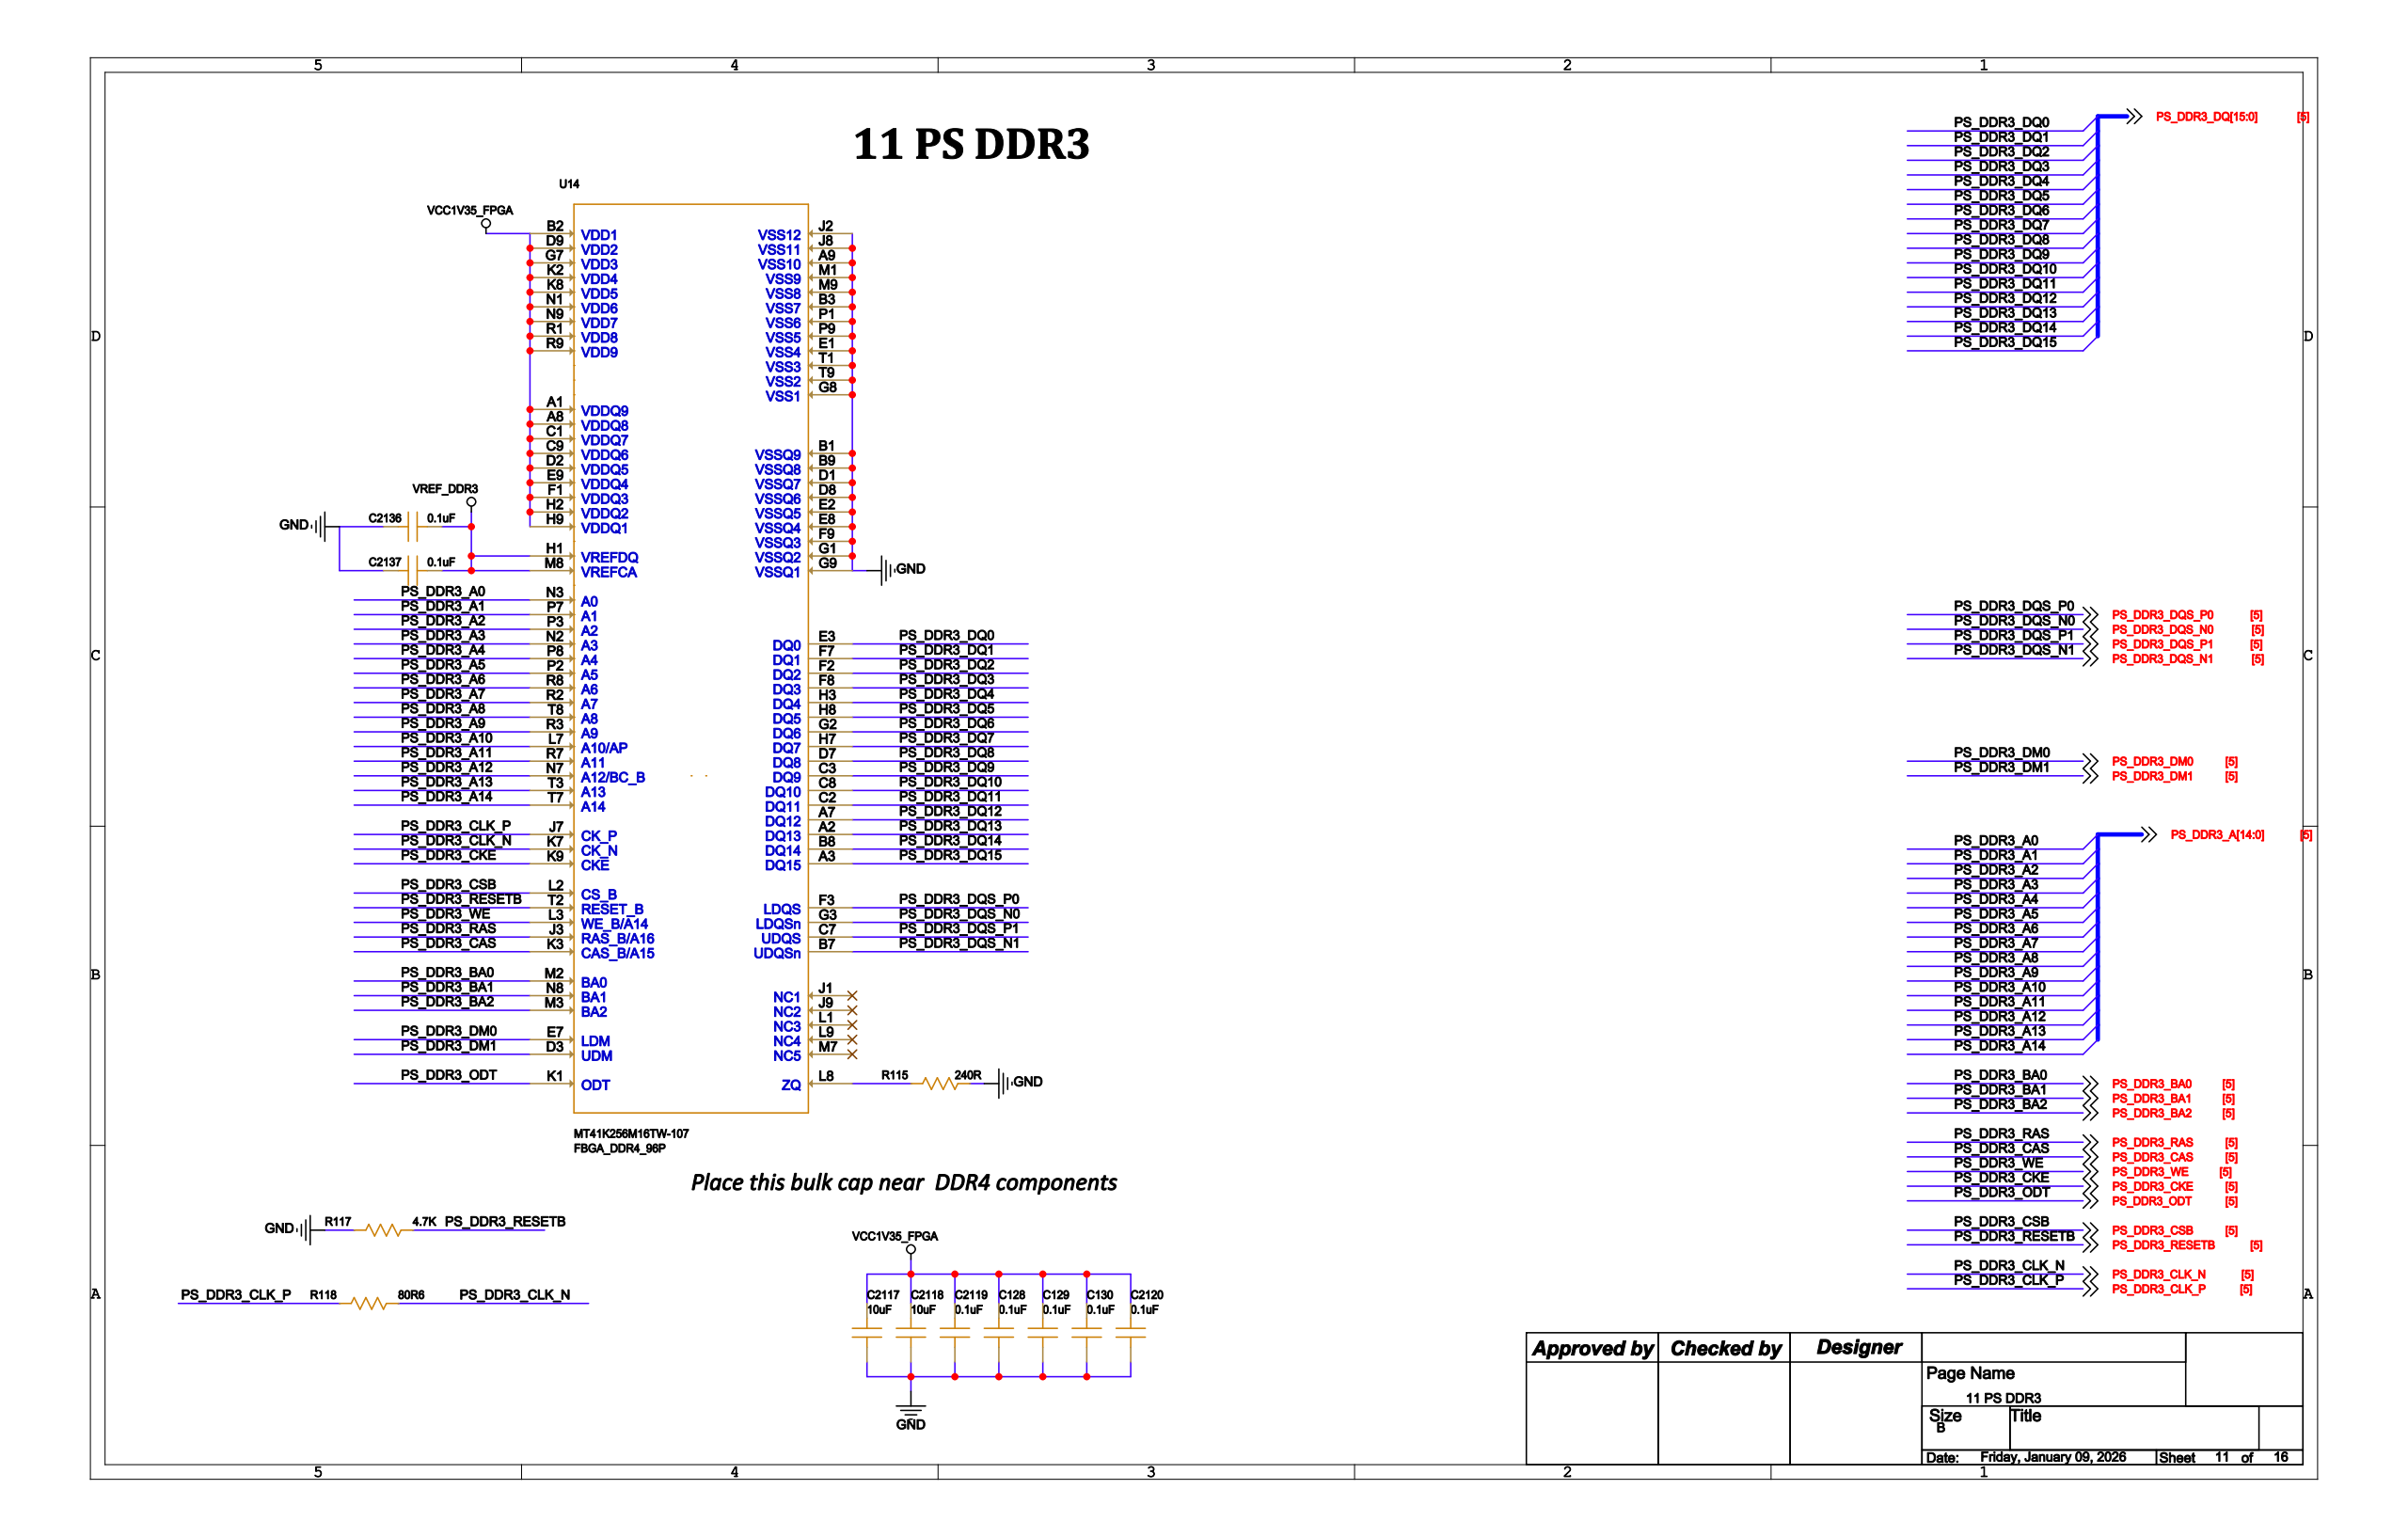Circuit board | Cadence Allegro | 442 parts | 326 nets | one sheet of the schematic
Parts on this sheet (reference | value | footprint):
C128 | 0.1uF | C0201
C129 | 0.1uF | C0201
C130 | 0.1uF | C0201
C2117 | 10uF | C0603
C2118 | 10uF | C0603
C2119 | 0.1uF | C0201
C2120 | 0.1uF | C0201
C2136 | 0.1uF | C0201
C2137 | 0.1uF | C0201
R115 | 240R | R0201
R117 | 4.7K | R0201
R118 | 80R6 | R0201
U14 | MT41K256M16TW-107 | FBGA_DDR4_96P
Nets of these parts (net: part-pin ...):
GND: C128-2 C129-2 C130-2 C2117-2 C2118-2 C2119-2 C2120-2 C2136-2 C2137-2 R115-2 R117-2 U14-A9 U14-B1 U14-B3 U14-B9 U14-D1 U14-D8 U14-E1 U14-E2 U14-E8 U14-F9 U14-G1 U14-G8 U14-G9 U14-J2 U14-J8 U14-M1 U14-M9 U14-P1 U14-P9 U14-T1 U14-T9
PS_DDR3_A0: U14-N3
PS_DDR3_A1: U14-P7
PS_DDR3_A10: U14-L7
PS_DDR3_A11: U14-R7
PS_DDR3_A12: U14-N7
PS_DDR3_A13: U14-T3
PS_DDR3_A14: U14-T7
PS_DDR3_A2: U14-P3
PS_DDR3_A3: U14-N2
PS_DDR3_A4: U14-P8
PS_DDR3_A5: U14-P2
PS_DDR3_A6: U14-R8
PS_DDR3_A7: U14-R2
PS_DDR3_A8: U14-T8
PS_DDR3_A9: U14-R3
PS_DDR3_BA0: U14-M2
PS_DDR3_BA1: U14-N8
PS_DDR3_BA2: U14-M3
PS_DDR3_CAS: U14-K3
PS_DDR3_CKE: U14-K9
PS_DDR3_CLK_N: R118-1 U14-K7
PS_DDR3_CLK_P: R118-2 U14-J7
PS_DDR3_CSB: U14-L2
PS_DDR3_DQ0: U14-E3
PS_DDR3_DQ1: U14-F7
PS_DDR3_DQ10: U14-C8
PS_DDR3_DQ11: U14-C2
PS_DDR3_DQ12: U14-A7
PS_DDR3_DQ13: U14-A2
PS_DDR3_DQ14: U14-B8
PS_DDR3_DQ15: U14-A3
PS_DDR3_DQ2: U14-F2
PS_DDR3_DQ3: U14-F8
PS_DDR3_DQ4: U14-H3
PS_DDR3_DQ5: U14-H8
PS_DDR3_DQ6: U14-G2
PS_DDR3_DQ7: U14-H7
PS_DDR3_DQ8: U14-D7
PS_DDR3_DQ9: U14-C3
PS_DDR3_DM0: U14-E7
PS_DDR3_DQS_P0: U14-F3
PS_DDR3_DQS_N0: U14-G3
PS_DDR3_ODT: U14-K1
PS_DDR3_RAS: U14-J3
PS_DDR3_RESETB: R117-1 U14-T2
PS_DDR3_DM1: U14-D3
PS_DDR3_DQS_P1: U14-C7
PS_DDR3_DQS_N1: U14-B7
VCC1V35_FPGA: C128-1 C129-1 C130-1 C2117-1 C2118-1 C2119-1 C2120-1 U14-A1 U14-A8 U14-B2 U14-C1 U14-C9 U14-D2 U14-D9 U14-E9 U14-F1 U14-G7 U14-H2 U14-H9 U14-K2 U14-K8 U14-N1 U14-N9 U14-R1 U14-R9
VREF_DDR3: C2136-1 C2137-1 U14-H1 U14-M8
PS_DDR3_WE: U14-L3
N49135745: R115-1 U14-L8